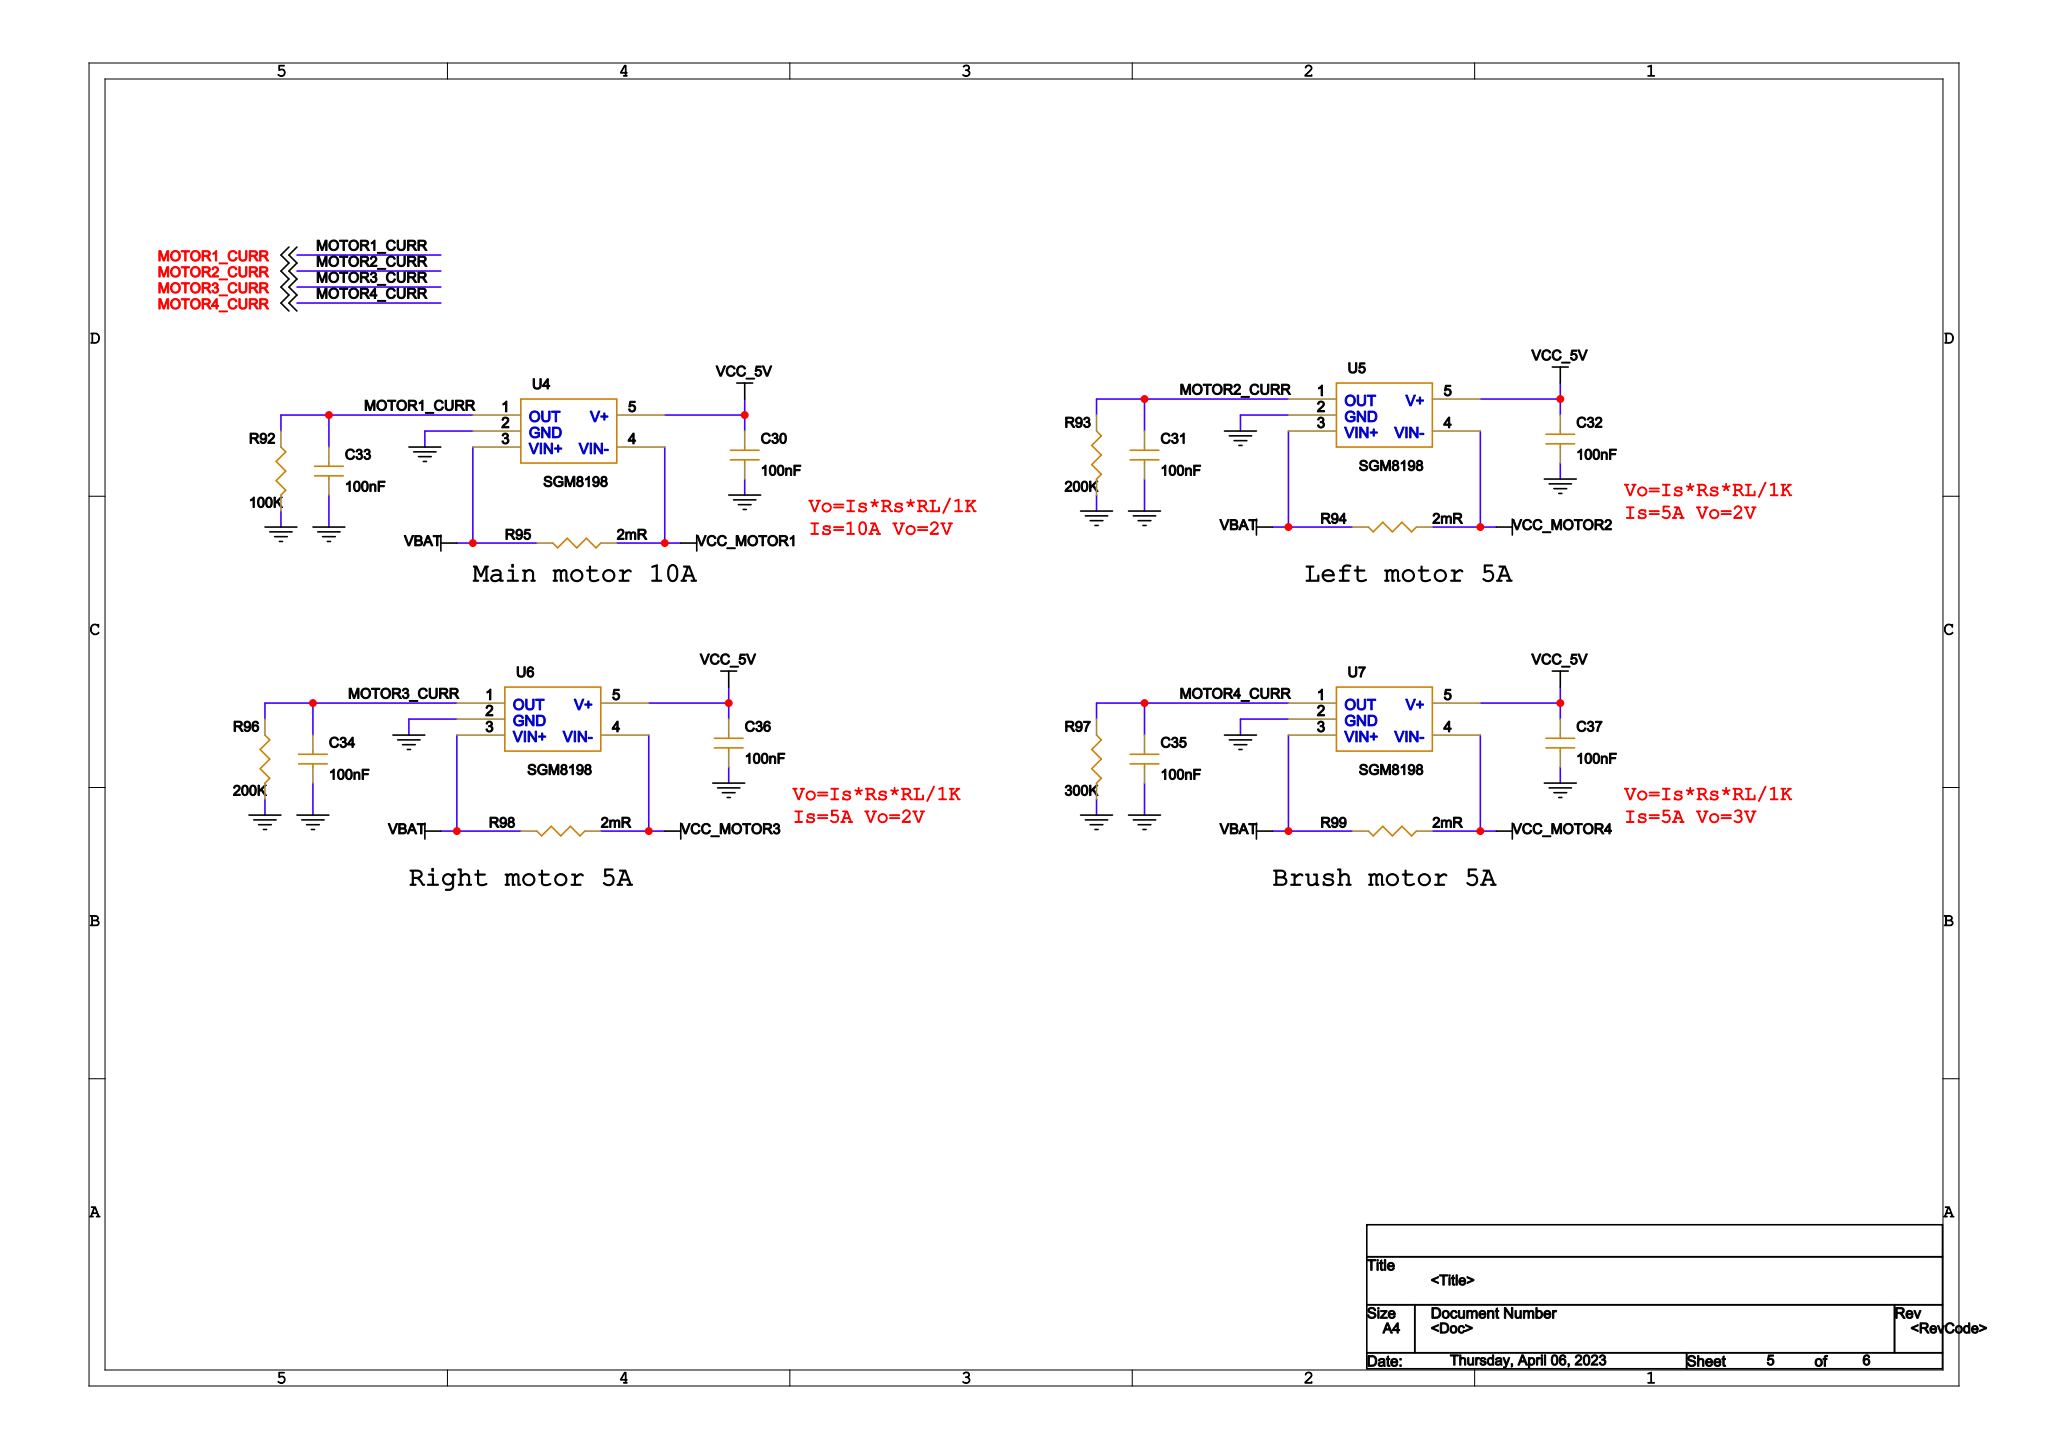Circuit board | Cadence Allegro | 278 parts | 154 nets | one sheet of the schematic
Parts on this sheet (reference | value | footprint):
C30 | 100nF | C0402
C31 | 100nF | C0402
C32 | 100nF | C0402
C33 | 100nF | C0402
C34 | 100nF | C0402
C35 | 100nF | C0402
C36 | 100nF | C0402
C37 | 100nF | C0402
R92 | 100K | R0402
R93 | 200K | R0402
R95 | 2mR | SMD3P2X6P4
R96 | 200K | R0402
R97 | 300K | R0402
R98 | 2mR | SMD3P2X6P4
R99 | 2mR | SMD3P2X6P4
U4 | SGM8198 | SOT-23_5
U5 | SGM8198 | SOT-23_5
Nets of these parts (net: part-pin ...):
GND: C30-1 C31-1 C32-1 C33-1 C34-1 C35-1 C36-1 C37-1 R92-2 R93-2 R96-2 R97-2 U4-2 U5-2
VCC_5V: C30-2 C32-2 C36-2 C37-2 U4-5 U5-5
MOTOR2_CURR: C31-2 R93-1 U5-1
MOTOR1_CURR: C33-2 R92-1 U4-1
MOTOR3_CURR: C34-2 R96-1
MOTOR4_CURR: C35-2 R97-1
VBAT: R95-2 R98-2 R99-2 U4-3 U5-3
VCC_MOTOR2: U5-4
VCC_MOTOR4: R99-1
VCC_MOTOR3: R98-1
VCC_MOTOR1: R95-1 U4-4